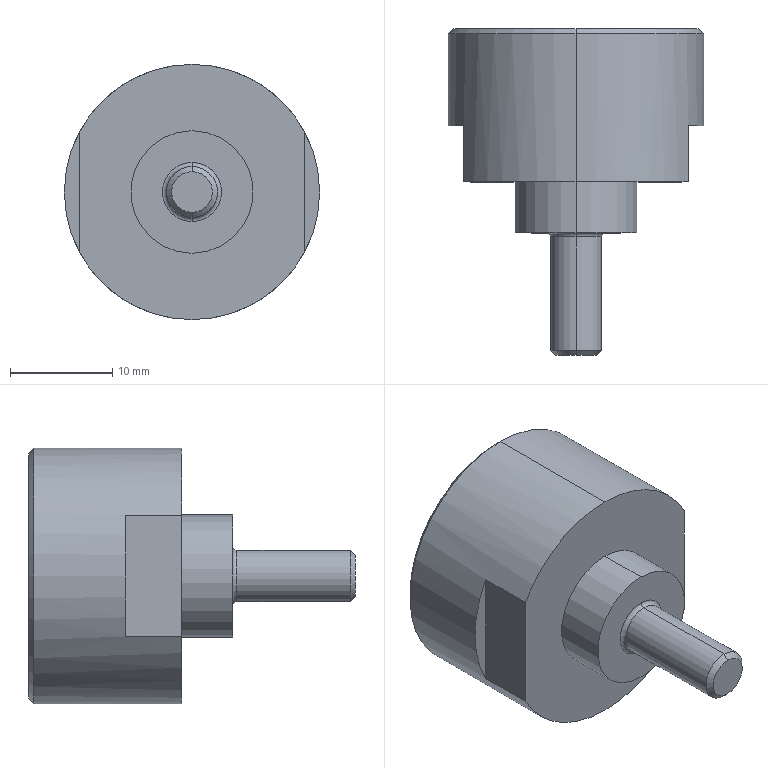Part | STEP file | OP10-157_seal rod (valve guide) | 1 solid | 40 faces | box 25 x 32 x 25 mm | volume 5292 mm3 | cylinder 18 | plane 12 | cone 8 | torus 2 | commonest cylinder face diameters 3 x8 5 x2 12 x2 19.1 x2 20.5 x2 25 x2